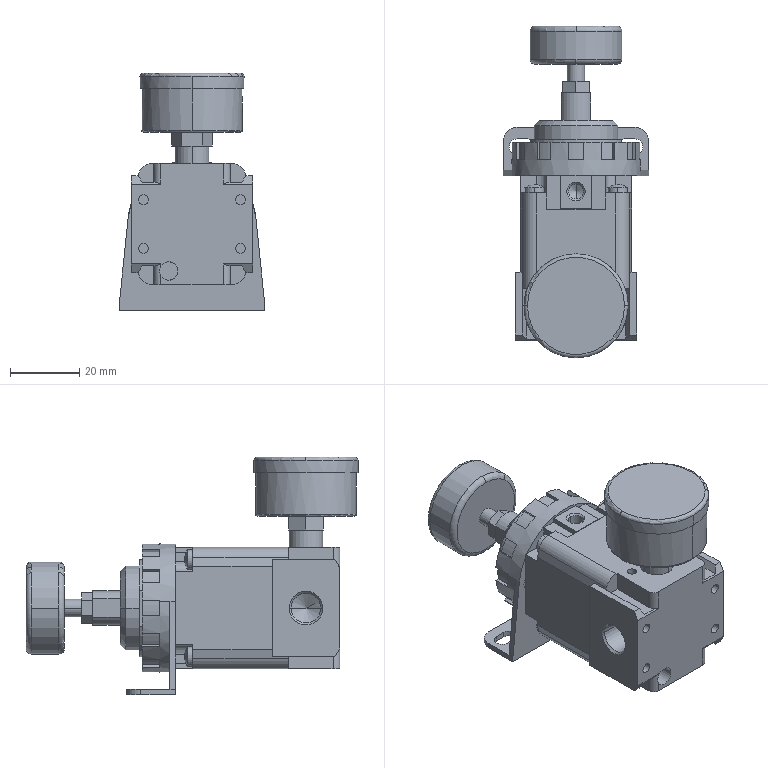Part | STEP file | IR1020-01BG-A_0_^Coding mechanism | 3 solids | 295 faces | box 42 x 95.7 x 68.5 mm | volume 83604 mm3 | plane 163 | cylinder 96 | cone 24 | torus 8 | sphere 4 | commonest cylinder face diameters 5 x12 35 x12 2.8 x8 5.6 x8 8 x6 8.566 x6